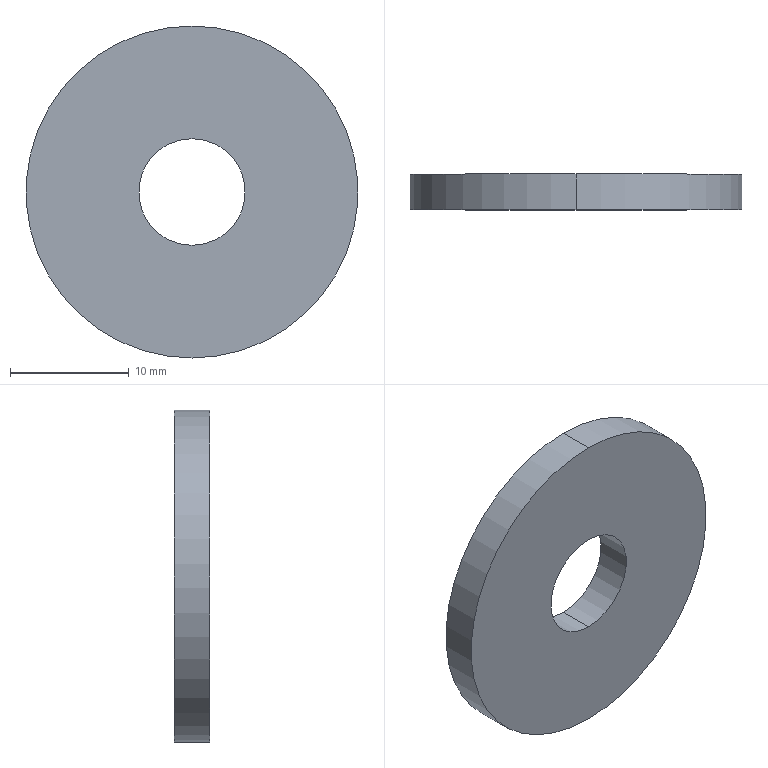Part | SolidWorks | features Revolution 1 | 1 solid | 6 faces | box 28 x 3 x 28 mm | volume 1656 mm3 | cylinder 4 | plane 2 | commonest cylinder face diameters 9 x2 28 x2
STEP:
#1=CARTESIAN_POINT('',(0.,11.645,-14.));
#2=VERTEX_POINT('',#1);
#3=CARTESIAN_POINT('',(0.,11.645,14.));
#4=VERTEX_POINT('',#3);
#5=CARTESIAN_POINT('',(0.,11.645,0.));
#6=DIRECTION('',(0.,-1.,0.));
#7=DIRECTION('',(0.,0.,-1.));
#8=AXIS2_PLACEMENT_3D('',#5,#6,#7);
#9=CIRCLE('',#8,14.);
#10=EDGE_CURVE('',#2,#4,#9,.T.);
#11=ORIENTED_EDGE('',*,*,#10,.T.);
#12=CARTESIAN_POINT('',(0.,8.645,14.));
#13=VERTEX_POINT('',#12);
#14=CARTESIAN_POINT('',(0.,0.,14.));
#15=DIRECTION('',(0.,-1.,0.));
#16=VECTOR('',#15,1000.);
#17=LINE('',#14,#16);
#18=EDGE_CURVE('',#4,#13,#17,.T.);
#19=ORIENTED_EDGE('',*,*,#18,.T.);
#20=CARTESIAN_POINT('',(0.,8.645,-14.));
#21=VERTEX_POINT('',#20);
#22=CARTESIAN_POINT('',(0.,8.645,0.));
#23=DIRECTION('',(0.,-1.,0.));
#24=DIRECTION('',(0.,0.,-1.));
#25=AXIS2_PLACEMENT_3D('',#22,#23,#24);
#26=CIRCLE('',#25,14.);
#27=EDGE_CURVE('',#21,#13,#26,.T.);
#28=ORIENTED_EDGE('',*,*,#27,.F.);
#29=CARTESIAN_POINT('',(0.,0.,-14.));
#30=DIRECTION('',(0.,-1.,0.));
#31=VECTOR('',#30,1000.);
#32=LINE('',#29,#31);
#33=EDGE_CURVE('',#2,#21,#32,.T.);
#34=ORIENTED_EDGE('',*,*,#33,.F.);
#35=EDGE_LOOP('',(#11,#19,#28,#34));
#36=FACE_OUTER_BOUND('',#35,.T.);
#37=CARTESIAN_POINT('',(0.,0.,0.));
#38=DIRECTION('',(0.,-1.,0.));
#39=DIRECTION('',(0.,0.,-1.));
#40=AXIS2_PLACEMENT_3D('',#37,#38,#39);
#41=CYLINDRICAL_SURFACE('',#40,14.);
#42=ADVANCED_FACE('',(#36),#41,.T.);
#43=CARTESIAN_POINT('',(0.,11.645,4.5));
#44=VERTEX_POINT('',#43);
#45=CARTESIAN_POINT('',(0.,11.645,-4.5));
#46=VERTEX_POINT('',#45);
#47=CARTESIAN_POINT('',(0.,11.645,0.));
#48=DIRECTION('',(0.,-1.,0.));
#49=DIRECTION('',(0.,0.,-1.));
#50=AXIS2_PLACEMENT_3D('',#47,#48,#49);
#51=CIRCLE('',#50,4.5);
#52=EDGE_CURVE('',#44,#46,#51,.T.);
#53=ORIENTED_EDGE('',*,*,#52,.F.);
#54=CARTESIAN_POINT('',(0.,8.645,4.5));
#55=VERTEX_POINT('',#54);
#56=CARTESIAN_POINT('',(0.,0.,4.5));
#57=DIRECTION('',(0.,-1.,0.));
#58=VECTOR('',#57,1000.);
#59=LINE('',#56,#58);
#60=EDGE_CURVE('',#44,#55,#59,.T.);
#61=ORIENTED_EDGE('',*,*,#60,.T.);
#62=CARTESIAN_POINT('',(0.,8.645,-4.5));
#63=VERTEX_POINT('',#62);
#64=CARTESIAN_POINT('',(0.,8.645,0.));
#65=DIRECTION('',(0.,-1.,0.));
#66=DIRECTION('',(0.,0.,-1.));
#67=AXIS2_PLACEMENT_3D('',#64,#65,#66);
#68=CIRCLE('',#67,4.5);
#69=EDGE_CURVE('',#55,#63,#68,.T.);
#70=ORIENTED_EDGE('',*,*,#69,.T.);
#71=CARTESIAN_POINT('',(0.,0.,-4.5));
#72=DIRECTION('',(0.,-1.,0.));
#73=VECTOR('',#72,1000.);
#74=LINE('',#71,#73);
#75=EDGE_CURVE('',#46,#63,#74,.T.);
#76=ORIENTED_EDGE('',*,*,#75,.F.);
#77=EDGE_LOOP('',(#53,#61,#70,#76));
#78=FACE_OUTER_BOUND('',#77,.T.);
#79=CARTESIAN_POINT('',(0.,0.,0.));
#80=DIRECTION('',(0.,-1.,0.));
#81=DIRECTION('',(0.,0.,-1.));
#82=AXIS2_PLACEMENT_3D('',#79,#80,#81);
#83=CYLINDRICAL_SURFACE('',#82,4.5);
#84=ADVANCED_FACE('',(#78),#83,.F.);
#85=ORIENTED_EDGE('',*,*,#60,.F.);
#86=CARTESIAN_POINT('',(0.,11.645,0.));
#87=DIRECTION('',(0.,-1.,0.));
#88=DIRECTION('',(0.,0.,-1.));
#89=AXIS2_PLACEMENT_3D('',#86,#87,#88);
#90=CIRCLE('',#89,4.5);
#91=EDGE_CURVE('',#46,#44,#90,.T.);
#92=ORIENTED_EDGE('',*,*,#91,.F.);
#93=ORIENTED_EDGE('',*,*,#75,.T.);
#94=CARTESIAN_POINT('',(0.,8.645,0.));
#95=DIRECTION('',(0.,-1.,0.));
#96=DIRECTION('',(0.,0.,-1.));
#97=AXIS2_PLACEMENT_3D('',#94,#95,#96);
#98=CIRCLE('',#97,4.5);
#99=EDGE_CURVE('',#63,#55,#98,.T.);
#100=ORIENTED_EDGE('',*,*,#99,.T.);
#101=EDGE_LOOP('',(#85,#92,#93,#100));
#102=FACE_OUTER_BOUND('',#101,.T.);
#103=CARTESIAN_POINT('',(0.,0.,0.));
#104=DIRECTION('',(0.,-1.,0.));
#105=DIRECTION('',(0.,0.,-1.));
#106=AXIS2_PLACEMENT_3D('',#103,#104,#105);
#107=CYLINDRICAL_SURFACE('',#106,4.5);
#108=ADVANCED_FACE('',(#102),#107,.F.);
#109=ORIENTED_EDGE('',*,*,#10,.F.);
#110=CARTESIAN_POINT('',(0.,11.645,0.));
#111=DIRECTION('',(0.,-1.,0.));
#112=DIRECTION('',(0.,0.,-1.));
#113=AXIS2_PLACEMENT_3D('',#110,#111,#112);
#114=CIRCLE('',#113,14.);
#115=EDGE_CURVE('',#4,#2,#114,.T.);
#116=ORIENTED_EDGE('',*,*,#115,.F.);
#117=EDGE_LOOP('',(#109,#116));
#118=FACE_OUTER_BOUND('',#117,.T.);
#119=ORIENTED_EDGE('',*,*,#91,.T.);
#120=ORIENTED_EDGE('',*,*,#52,.T.);
#121=EDGE_LOOP('',(#119,#120));
#122=FACE_BOUND('',#121,.T.);
#123=CARTESIAN_POINT('',(-4.5,11.645,0.));
#124=DIRECTION('',(0.,-1.,0.));
#125=DIRECTION('',(0.,0.,-1.));
#126=AXIS2_PLACEMENT_3D('',#123,#124,#125);
#127=PLANE('',#126);
#128=ADVANCED_FACE('',(#118,#122),#127,.F.);
#129=ORIENTED_EDGE('',*,*,#18,.F.);
#130=ORIENTED_EDGE('',*,*,#115,.T.);
#131=ORIENTED_EDGE('',*,*,#33,.T.);
#132=CARTESIAN_POINT('',(0.,8.645,0.));
#133=DIRECTION('',(0.,-1.,0.));
#134=DIRECTION('',(0.,0.,-1.));
#135=AXIS2_PLACEMENT_3D('',#132,#133,#134);
#136=CIRCLE('',#135,14.);
#137=EDGE_CURVE('',#13,#21,#136,.T.);
#138=ORIENTED_EDGE('',*,*,#137,.F.);
#139=EDGE_LOOP('',(#129,#130,#131,#138));
#140=FACE_OUTER_BOUND('',#139,.T.);
#141=CARTESIAN_POINT('',(0.,0.,0.));
#142=DIRECTION('',(0.,-1.,0.));
#143=DIRECTION('',(0.,0.,-1.));
#144=AXIS2_PLACEMENT_3D('',#141,#142,#143);
#145=CYLINDRICAL_SURFACE('',#144,14.);
#146=ADVANCED_FACE('',(#140),#145,.T.);
#147=ORIENTED_EDGE('',*,*,#99,.F.);
#148=ORIENTED_EDGE('',*,*,#69,.F.);
#149=EDGE_LOOP('',(#147,#148));
#150=FACE_BOUND('',#149,.T.);
#151=ORIENTED_EDGE('',*,*,#27,.T.);
#152=ORIENTED_EDGE('',*,*,#137,.T.);
#153=EDGE_LOOP('',(#151,#152));
#154=FACE_OUTER_BOUND('',#153,.T.);
#155=CARTESIAN_POINT('',(-4.5,8.645,0.));
#156=DIRECTION('',(0.,1.,0.));
#157=DIRECTION('',(0.,0.,1.));
#158=AXIS2_PLACEMENT_3D('',#155,#156,#157);
#159=PLANE('',#158);
#160=ADVANCED_FACE('',(#150,#154),#159,.F.);
#161=CLOSED_SHELL('',(#42,#84,#108,#128,#146,#160));
#162=MANIFOLD_SOLID_BREP('',#161);
#163=CARTESIAN_POINT('',(0.,0.,0.));
#164=DIRECTION('',(0.,0.,1.));
#165=DIRECTION('',(1.,0.,0.));
#166=AXIS2_PLACEMENT_3D('',#163,#164,#165);
#167=(LENGTH_UNIT()NAMED_UNIT(*)SI_UNIT(.MILLI.,.METRE.));
#168=UNCERTAINTY_MEASURE_WITH_UNIT(LENGTH_MEASURE(0.00001),#167,'','');
#169=(NAMED_UNIT(*)PLANE_ANGLE_UNIT()SI_UNIT($,.RADIAN.));
#170=(NAMED_UNIT(*)SI_UNIT($,.STERADIAN.)SOLID_ANGLE_UNIT());
#171=(GEOMETRIC_REPRESENTATION_CONTEXT(3)GLOBAL_UNCERTAINTY_ASSIGNED_CONTEXT((#168))GLOBAL_UNIT_ASSIGNED_CONTEXT((#167,#169,#170))REPRESENTATION_CONTEXT('',''));
#172=ADVANCED_BREP_SHAPE_REPRESENTATION('',(#162,#166),#171);